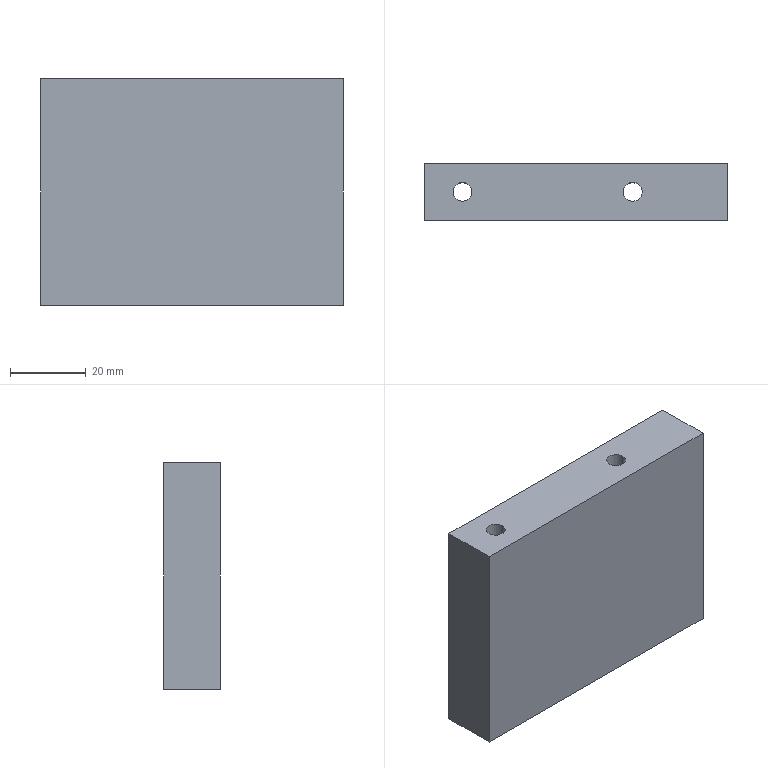Part | STEP file | PN_0025 | 1 solid | 10 faces | box 80 x 15 x 60 mm | volume 69644 mm3 | plane 6 | cylinder 4 | commonest cylinder face diameters 5 x4
STEP:
#1=CARTESIAN_POINT('',(0.,0.,0.));
#2=DIRECTION('',(0.,0.,1.));
#3=DIRECTION('',(1.,0.,0.));
#4=AXIS2_PLACEMENT_3D('',#1,#2,#3);
#5=CARTESIAN_POINT('',(-27.5,0.,-30.));
#6=VERTEX_POINT('',#5);
#7=CARTESIAN_POINT('',(-27.5,0.,30.));
#8=VERTEX_POINT('',#7);
#9=CARTESIAN_POINT('',(-27.5,0.,30.));
#10=DIRECTION('',(0.,0.,1.));
#11=VECTOR('',#10,1.);
#12=LINE('',#9,#11);
#13=CARTESIAN_POINT('',(-30.,0.,30.));
#14=DIRECTION('',(0.,0.,1.));
#15=DIRECTION('',(1.,0.,0.));
#16=AXIS2_PLACEMENT_3D('',#13,#14,#15);
#17=CYLINDRICAL_SURFACE('',#16,2.5);
#18=CARTESIAN_POINT('',(6.283,0.));
#19=DIRECTION('',(0.,1.));
#20=VECTOR('',#19,1.);
#21=LINE('',#18,#20);
#22=(GEOMETRIC_REPRESENTATION_CONTEXT(2)PARAMETRIC_REPRESENTATION_CONTEXT()REPRESENTATION_CONTEXT('',''));
#23=DEFINITIONAL_REPRESENTATION('',(#21),#22);
#24=PCURVE('',#17,#23);
#25=CARTESIAN_POINT('',(-30.,0.,30.));
#26=DIRECTION('',(0.,0.,1.));
#27=DIRECTION('',(1.,0.,0.));
#28=AXIS2_PLACEMENT_3D('',#25,#26,#27);
#29=CYLINDRICAL_SURFACE('',#28,2.5);
#30=CARTESIAN_POINT('',(0.,0.));
#31=DIRECTION('',(0.,1.));
#32=VECTOR('',#31,1.);
#33=LINE('',#30,#32);
#34=(GEOMETRIC_REPRESENTATION_CONTEXT(2)PARAMETRIC_REPRESENTATION_CONTEXT()REPRESENTATION_CONTEXT('',''));
#35=DEFINITIONAL_REPRESENTATION('',(#33),#34);
#36=PCURVE('',#29,#35);
#37=SURFACE_CURVE('',#12,(#24,#36),.PCURVE_S1.);
#38=EDGE_CURVE('',#6,#8,#37,.T.);
#39=ORIENTED_EDGE('',*,*,#38,.T.);
#40=CARTESIAN_POINT('',(-32.5,0.,30.));
#41=VERTEX_POINT('',#40);
#42=CARTESIAN_POINT('',(-30.,0.,30.));
#43=DIRECTION('',(0.,0.,1.));
#44=DIRECTION('',(1.,0.,0.));
#45=AXIS2_PLACEMENT_3D('',#42,#43,#44);
#46=CIRCLE('',#45,2.5);
#47=CARTESIAN_POINT('',(0.,0.));
#48=DIRECTION('',(1.,0.));
#49=VECTOR('',#48,1.);
#50=LINE('',#47,#49);
#51=(GEOMETRIC_REPRESENTATION_CONTEXT(2)PARAMETRIC_REPRESENTATION_CONTEXT()REPRESENTATION_CONTEXT('',''));
#52=DEFINITIONAL_REPRESENTATION('',(#50),#51);
#53=PCURVE('',#17,#52);
#54=CARTESIAN_POINT('',(-40.,7.5,30.));
#55=DIRECTION('',(0.,0.,-1.));
#56=DIRECTION('',(-1.,0.,0.));
#57=AXIS2_PLACEMENT_3D('',#54,#55,#56);
#58=PLANE('',#57);
#59=CARTESIAN_POINT('',(-12.5,-7.5));
#60=CARTESIAN_POINT('',(-12.5,-3.17));
#61=CARTESIAN_POINT('',(-8.75,-5.335));
#62=CARTESIAN_POINT('',(-5.,-7.5));
#63=CARTESIAN_POINT('',(-8.75,-9.665));
#64=CARTESIAN_POINT('',(-12.5,-11.83));
#65=CARTESIAN_POINT('',(-12.5,-7.5));
#66=(BOUNDED_CURVE()B_SPLINE_CURVE(2,(#59,#60,#61,#62,#63,#64,#65),.UNSPECIFIED.,.T.,.F.)B_SPLINE_CURVE_WITH_KNOTS((1,2,2,2,2,1),(-2.094,0.,2.094,4.189,6.283,8.378),.UNSPECIFIED.)CURVE()GEOMETRIC_REPRESENTATION_ITEM()RATIONAL_B_SPLINE_CURVE((1.,0.5,1.,0.5,1.,0.5,1.))REPRESENTATION_ITEM(''));
#67=(GEOMETRIC_REPRESENTATION_CONTEXT(2)PARAMETRIC_REPRESENTATION_CONTEXT()REPRESENTATION_CONTEXT('',''));
#68=DEFINITIONAL_REPRESENTATION('',(#66),#67);
#69=PCURVE('',#58,#68);
#70=SURFACE_CURVE('',#46,(#53,#69),.PCURVE_S1.);
#71=EDGE_CURVE('',#41,#8,#70,.T.);
#72=ORIENTED_EDGE('',*,*,#71,.F.);
#73=CARTESIAN_POINT('',(-32.5,0.,-30.));
#74=VERTEX_POINT('',#73);
#75=CARTESIAN_POINT('',(-32.5,0.,30.));
#76=DIRECTION('',(0.,0.,1.));
#77=VECTOR('',#76,1.);
#78=LINE('',#75,#77);
#79=CARTESIAN_POINT('',(3.142,0.));
#80=DIRECTION('',(0.,1.));
#81=VECTOR('',#80,1.);
#82=LINE('',#79,#81);
#83=(GEOMETRIC_REPRESENTATION_CONTEXT(2)PARAMETRIC_REPRESENTATION_CONTEXT()REPRESENTATION_CONTEXT('',''));
#84=DEFINITIONAL_REPRESENTATION('',(#82),#83);
#85=PCURVE('',#17,#84);
#86=CARTESIAN_POINT('',(3.142,0.));
#87=DIRECTION('',(0.,1.));
#88=VECTOR('',#87,1.);
#89=LINE('',#86,#88);
#90=(GEOMETRIC_REPRESENTATION_CONTEXT(2)PARAMETRIC_REPRESENTATION_CONTEXT()REPRESENTATION_CONTEXT('',''));
#91=DEFINITIONAL_REPRESENTATION('',(#89),#90);
#92=PCURVE('',#29,#91);
#93=SURFACE_CURVE('',#78,(#85,#92),.PCURVE_S1.);
#94=EDGE_CURVE('',#74,#41,#93,.T.);
#95=ORIENTED_EDGE('',*,*,#94,.F.);
#96=CARTESIAN_POINT('',(-30.,0.,-30.));
#97=DIRECTION('',(0.,0.,1.));
#98=DIRECTION('',(1.,0.,0.));
#99=AXIS2_PLACEMENT_3D('',#96,#97,#98);
#100=CIRCLE('',#99,2.5);
#101=CARTESIAN_POINT('',(0.,-60.));
#102=DIRECTION('',(1.,0.));
#103=VECTOR('',#102,1.);
#104=LINE('',#101,#103);
#105=(GEOMETRIC_REPRESENTATION_CONTEXT(2)PARAMETRIC_REPRESENTATION_CONTEXT()REPRESENTATION_CONTEXT('',''));
#106=DEFINITIONAL_REPRESENTATION('',(#104),#105);
#107=PCURVE('',#17,#106);
#108=CARTESIAN_POINT('',(-40.,7.5,-30.));
#109=DIRECTION('',(0.,0.,1.));
#110=DIRECTION('',(1.,0.,0.));
#111=AXIS2_PLACEMENT_3D('',#108,#109,#110);
#112=PLANE('',#111);
#113=CARTESIAN_POINT('',(10.,-7.5));
#114=DIRECTION('',(1.,0.));
#115=AXIS2_PLACEMENT_2D('',#113,#114);
#116=CIRCLE('',#115,2.5);
#117=(GEOMETRIC_REPRESENTATION_CONTEXT(2)PARAMETRIC_REPRESENTATION_CONTEXT()REPRESENTATION_CONTEXT('',''));
#118=DEFINITIONAL_REPRESENTATION('',(#116),#117);
#119=PCURVE('',#112,#118);
#120=SURFACE_CURVE('',#100,(#107,#119),.PCURVE_S1.);
#121=EDGE_CURVE('',#74,#6,#120,.T.);
#122=ORIENTED_EDGE('',*,*,#121,.T.);
#123=EDGE_LOOP('',(#39,#72,#95,#122));
#124=FACE_BOUND('',#123,.F.);
#125=ADVANCED_FACE('',(#124),#17,.F.);
#126=CARTESIAN_POINT('',(17.5,0.,-30.));
#127=VERTEX_POINT('',#126);
#128=CARTESIAN_POINT('',(17.5,0.,30.));
#129=VERTEX_POINT('',#128);
#130=CARTESIAN_POINT('',(17.5,0.,30.));
#131=DIRECTION('',(0.,0.,1.));
#132=VECTOR('',#131,1.);
#133=LINE('',#130,#132);
#134=CARTESIAN_POINT('',(15.,0.,30.));
#135=DIRECTION('',(0.,0.,1.));
#136=DIRECTION('',(1.,0.,0.));
#137=AXIS2_PLACEMENT_3D('',#134,#135,#136);
#138=CYLINDRICAL_SURFACE('',#137,2.5);
#139=CARTESIAN_POINT('',(6.283,0.));
#140=DIRECTION('',(0.,1.));
#141=VECTOR('',#140,1.);
#142=LINE('',#139,#141);
#143=(GEOMETRIC_REPRESENTATION_CONTEXT(2)PARAMETRIC_REPRESENTATION_CONTEXT()REPRESENTATION_CONTEXT('',''));
#144=DEFINITIONAL_REPRESENTATION('',(#142),#143);
#145=PCURVE('',#138,#144);
#146=CARTESIAN_POINT('',(15.,0.,30.));
#147=DIRECTION('',(0.,0.,1.));
#148=DIRECTION('',(1.,0.,0.));
#149=AXIS2_PLACEMENT_3D('',#146,#147,#148);
#150=CYLINDRICAL_SURFACE('',#149,2.5);
#151=CARTESIAN_POINT('',(0.,0.));
#152=DIRECTION('',(0.,1.));
#153=VECTOR('',#152,1.);
#154=LINE('',#151,#153);
#155=(GEOMETRIC_REPRESENTATION_CONTEXT(2)PARAMETRIC_REPRESENTATION_CONTEXT()REPRESENTATION_CONTEXT('',''));
#156=DEFINITIONAL_REPRESENTATION('',(#154),#155);
#157=PCURVE('',#150,#156);
#158=SURFACE_CURVE('',#133,(#145,#157),.PCURVE_S1.);
#159=EDGE_CURVE('',#127,#129,#158,.T.);
#160=ORIENTED_EDGE('',*,*,#159,.T.);
#161=CARTESIAN_POINT('',(12.5,0.,30.));
#162=VERTEX_POINT('',#161);
#163=CARTESIAN_POINT('',(15.,0.,30.));
#164=DIRECTION('',(0.,0.,1.));
#165=DIRECTION('',(1.,0.,0.));
#166=AXIS2_PLACEMENT_3D('',#163,#164,#165);
#167=CIRCLE('',#166,2.5);
#168=CARTESIAN_POINT('',(0.,0.));
#169=DIRECTION('',(1.,0.));
#170=VECTOR('',#169,1.);
#171=LINE('',#168,#170);
#172=(GEOMETRIC_REPRESENTATION_CONTEXT(2)PARAMETRIC_REPRESENTATION_CONTEXT()REPRESENTATION_CONTEXT('',''));
#173=DEFINITIONAL_REPRESENTATION('',(#171),#172);
#174=PCURVE('',#138,#173);
#175=CARTESIAN_POINT('',(-57.5,-7.5));
#176=CARTESIAN_POINT('',(-57.5,-3.17));
#177=CARTESIAN_POINT('',(-53.75,-5.335));
#178=CARTESIAN_POINT('',(-50.,-7.5));
#179=CARTESIAN_POINT('',(-53.75,-9.665));
#180=CARTESIAN_POINT('',(-57.5,-11.83));
#181=CARTESIAN_POINT('',(-57.5,-7.5));
#182=(BOUNDED_CURVE()B_SPLINE_CURVE(2,(#175,#176,#177,#178,#179,#180,#181),.UNSPECIFIED.,.T.,.F.)B_SPLINE_CURVE_WITH_KNOTS((1,2,2,2,2,1),(-2.094,0.,2.094,4.189,6.283,8.378),.UNSPECIFIED.)CURVE()GEOMETRIC_REPRESENTATION_ITEM()RATIONAL_B_SPLINE_CURVE((1.,0.5,1.,0.5,1.,0.5,1.))REPRESENTATION_ITEM(''));
#183=(GEOMETRIC_REPRESENTATION_CONTEXT(2)PARAMETRIC_REPRESENTATION_CONTEXT()REPRESENTATION_CONTEXT('',''));
#184=DEFINITIONAL_REPRESENTATION('',(#182),#183);
#185=PCURVE('',#58,#184);
#186=SURFACE_CURVE('',#167,(#174,#185),.PCURVE_S1.);
#187=EDGE_CURVE('',#162,#129,#186,.T.);
#188=ORIENTED_EDGE('',*,*,#187,.F.);
#189=CARTESIAN_POINT('',(12.5,0.,-30.));
#190=VERTEX_POINT('',#189);
#191=CARTESIAN_POINT('',(12.5,0.,30.));
#192=DIRECTION('',(0.,0.,1.));
#193=VECTOR('',#192,1.);
#194=LINE('',#191,#193);
#195=CARTESIAN_POINT('',(3.142,0.));
#196=DIRECTION('',(0.,1.));
#197=VECTOR('',#196,1.);
#198=LINE('',#195,#197);
#199=(GEOMETRIC_REPRESENTATION_CONTEXT(2)PARAMETRIC_REPRESENTATION_CONTEXT()REPRESENTATION_CONTEXT('',''));
#200=DEFINITIONAL_REPRESENTATION('',(#198),#199);
#201=PCURVE('',#138,#200);
#202=CARTESIAN_POINT('',(3.142,0.));
#203=DIRECTION('',(0.,1.));
#204=VECTOR('',#203,1.);
#205=LINE('',#202,#204);
#206=(GEOMETRIC_REPRESENTATION_CONTEXT(2)PARAMETRIC_REPRESENTATION_CONTEXT()REPRESENTATION_CONTEXT('',''));
#207=DEFINITIONAL_REPRESENTATION('',(#205),#206);
#208=PCURVE('',#150,#207);
#209=SURFACE_CURVE('',#194,(#201,#208),.PCURVE_S1.);
#210=EDGE_CURVE('',#190,#162,#209,.T.);
#211=ORIENTED_EDGE('',*,*,#210,.F.);
#212=CARTESIAN_POINT('',(15.,0.,-30.));
#213=DIRECTION('',(0.,0.,1.));
#214=DIRECTION('',(1.,0.,0.));
#215=AXIS2_PLACEMENT_3D('',#212,#213,#214);
#216=CIRCLE('',#215,2.5);
#217=CARTESIAN_POINT('',(0.,-60.));
#218=DIRECTION('',(1.,0.));
#219=VECTOR('',#218,1.);
#220=LINE('',#217,#219);
#221=(GEOMETRIC_REPRESENTATION_CONTEXT(2)PARAMETRIC_REPRESENTATION_CONTEXT()REPRESENTATION_CONTEXT('',''));
#222=DEFINITIONAL_REPRESENTATION('',(#220),#221);
#223=PCURVE('',#138,#222);
#224=CARTESIAN_POINT('',(55.,-7.5));
#225=DIRECTION('',(1.,0.));
#226=AXIS2_PLACEMENT_2D('',#224,#225);
#227=CIRCLE('',#226,2.5);
#228=(GEOMETRIC_REPRESENTATION_CONTEXT(2)PARAMETRIC_REPRESENTATION_CONTEXT()REPRESENTATION_CONTEXT('',''));
#229=DEFINITIONAL_REPRESENTATION('',(#227),#228);
#230=PCURVE('',#112,#229);
#231=SURFACE_CURVE('',#216,(#223,#230),.PCURVE_S1.);
#232=EDGE_CURVE('',#190,#127,#231,.T.);
#233=ORIENTED_EDGE('',*,*,#232,.T.);
#234=EDGE_LOOP('',(#160,#188,#211,#233));
#235=FACE_BOUND('',#234,.F.);
#236=ADVANCED_FACE('',(#235),#138,.F.);
#237=CARTESIAN_POINT('',(40.,-7.5,30.));
#238=VERTEX_POINT('',#237);
#239=CARTESIAN_POINT('',(40.,-7.5,-30.));
#240=VERTEX_POINT('',#239);
#241=CARTESIAN_POINT('',(40.,-7.5,-30.));
#242=DIRECTION('',(0.,0.,-1.));
#243=VECTOR('',#242,1.);
#244=LINE('',#241,#243);
#245=CARTESIAN_POINT('',(40.,7.5,-30.));
#246=DIRECTION('',(-1.,0.,0.));
#247=DIRECTION('',(0.,0.,1.));
#248=AXIS2_PLACEMENT_3D('',#245,#246,#247);
#249=PLANE('',#248);
#250=CARTESIAN_POINT('',(0.,-15.));
#251=DIRECTION('',(-1.,0.));
#252=VECTOR('',#251,1.);
#253=LINE('',#250,#252);
#254=(GEOMETRIC_REPRESENTATION_CONTEXT(2)PARAMETRIC_REPRESENTATION_CONTEXT()REPRESENTATION_CONTEXT('',''));
#255=DEFINITIONAL_REPRESENTATION('',(#253),#254);
#256=PCURVE('',#249,#255);
#257=CARTESIAN_POINT('',(0.,-7.5,0.));
#258=DIRECTION('',(0.,1.,0.));
#259=DIRECTION('',(0.,0.,1.));
#260=AXIS2_PLACEMENT_3D('',#257,#258,#259);
#261=PLANE('',#260);
#262=CARTESIAN_POINT('',(-30.,40.));
#263=DIRECTION('',(-1.,0.));
#264=VECTOR('',#263,1.);
#265=LINE('',#262,#264);
#266=(GEOMETRIC_REPRESENTATION_CONTEXT(2)PARAMETRIC_REPRESENTATION_CONTEXT()REPRESENTATION_CONTEXT('',''));
#267=DEFINITIONAL_REPRESENTATION('',(#265),#266);
#268=PCURVE('',#261,#267);
#269=SURFACE_CURVE('',#244,(#256,#268),.PCURVE_S1.);
#270=EDGE_CURVE('',#238,#240,#269,.T.);
#271=ORIENTED_EDGE('',*,*,#270,.T.);
#272=CARTESIAN_POINT('',(40.,7.5,-30.));
#273=VERTEX_POINT('',#272);
#274=CARTESIAN_POINT('',(40.,7.5,-30.));
#275=DIRECTION('',(0.,-1.,0.));
#276=VECTOR('',#275,1.);
#277=LINE('',#274,#276);
#278=CARTESIAN_POINT('',(0.,0.));
#279=DIRECTION('',(0.,-1.));
#280=VECTOR('',#279,1.);
#281=LINE('',#278,#280);
#282=(GEOMETRIC_REPRESENTATION_CONTEXT(2)PARAMETRIC_REPRESENTATION_CONTEXT()REPRESENTATION_CONTEXT('',''));
#283=DEFINITIONAL_REPRESENTATION('',(#281),#282);
#284=PCURVE('',#249,#283);
#285=CARTESIAN_POINT('',(80.,0.));
#286=DIRECTION('',(0.,-1.));
#287=VECTOR('',#286,1.);
#288=LINE('',#285,#287);
#289=(GEOMETRIC_REPRESENTATION_CONTEXT(2)PARAMETRIC_REPRESENTATION_CONTEXT()REPRESENTATION_CONTEXT('',''));
#290=DEFINITIONAL_REPRESENTATION('',(#288),#289);
#291=PCURVE('',#112,#290);
#292=SURFACE_CURVE('',#277,(#284,#291),.PCURVE_S1.);
#293=EDGE_CURVE('',#273,#240,#292,.T.);
#294=ORIENTED_EDGE('',*,*,#293,.F.);
#295=CARTESIAN_POINT('',(40.,7.5,30.));
#296=VERTEX_POINT('',#295);
#297=CARTESIAN_POINT('',(40.,7.5,-30.));
#298=DIRECTION('',(0.,0.,-1.));
#299=VECTOR('',#298,1.);
#300=LINE('',#297,#299);
#301=CARTESIAN_POINT('',(0.,0.));
#302=DIRECTION('',(-1.,0.));
#303=VECTOR('',#302,1.);
#304=LINE('',#301,#303);
#305=(GEOMETRIC_REPRESENTATION_CONTEXT(2)PARAMETRIC_REPRESENTATION_CONTEXT()REPRESENTATION_CONTEXT('',''));
#306=DEFINITIONAL_REPRESENTATION('',(#304),#305);
#307=PCURVE('',#249,#306);
#308=CARTESIAN_POINT('',(0.,7.5,0.));
#309=DIRECTION('',(0.,1.,0.));
#310=DIRECTION('',(0.,0.,1.));
#311=AXIS2_PLACEMENT_3D('',#308,#309,#310);
#312=PLANE('',#311);
#313=CARTESIAN_POINT('',(-30.,40.));
#314=DIRECTION('',(-1.,0.));
#315=VECTOR('',#314,1.);
#316=LINE('',#313,#315);
#317=(GEOMETRIC_REPRESENTATION_CONTEXT(2)PARAMETRIC_REPRESENTATION_CONTEXT()REPRESENTATION_CONTEXT('',''));
#318=DEFINITIONAL_REPRESENTATION('',(#316),#317);
#319=PCURVE('',#312,#318);
#320=SURFACE_CURVE('',#300,(#307,#319),.PCURVE_S1.);
#321=EDGE_CURVE('',#296,#273,#320,.T.);
#322=ORIENTED_EDGE('',*,*,#321,.F.);
#323=CARTESIAN_POINT('',(40.,7.5,30.));
#324=DIRECTION('',(0.,-1.,0.));
#325=VECTOR('',#324,1.);
#326=LINE('',#323,#325);
#327=CARTESIAN_POINT('',(60.,0.));
#328=DIRECTION('',(0.,-1.));
#329=VECTOR('',#328,1.);
#330=LINE('',#327,#329);
#331=(GEOMETRIC_REPRESENTATION_CONTEXT(2)PARAMETRIC_REPRESENTATION_CONTEXT()REPRESENTATION_CONTEXT('',''));
#332=DEFINITIONAL_REPRESENTATION('',(#330),#331);
#333=PCURVE('',#249,#332);
#334=CARTESIAN_POINT('',(-80.,0.));
#335=DIRECTION('',(0.,-1.));
#336=VECTOR('',#335,1.);
#337=LINE('',#334,#336);
#338=(GEOMETRIC_REPRESENTATION_CONTEXT(2)PARAMETRIC_REPRESENTATION_CONTEXT()REPRESENTATION_CONTEXT('',''));
#339=DEFINITIONAL_REPRESENTATION('',(#337),#338);
#340=PCURVE('',#58,#339);
#341=SURFACE_CURVE('',#326,(#333,#340),.PCURVE_S1.);
#342=EDGE_CURVE('',#296,#238,#341,.T.);
#343=ORIENTED_EDGE('',*,*,#342,.T.);
#344=EDGE_LOOP('',(#271,#294,#322,#343));
#345=FACE_BOUND('',#344,.T.);
#346=ADVANCED_FACE('',(#345),#249,.F.);
#347=CARTESIAN_POINT('',(-30.,0.,-30.));
#348=DIRECTION('',(0.,0.,1.));
#349=DIRECTION('',(1.,0.,0.));
#350=AXIS2_PLACEMENT_3D('',#347,#348,#349);
#351=CIRCLE('',#350,2.5);
#352=CARTESIAN_POINT('',(10.,-7.5));
#353=DIRECTION('',(1.,0.));
#354=AXIS2_PLACEMENT_2D('',#352,#353);
#355=CIRCLE('',#354,2.5);
#356=(GEOMETRIC_REPRESENTATION_CONTEXT(2)PARAMETRIC_REPRESENTATION_CONTEXT()REPRESENTATION_CONTEXT('',''));
#357=DEFINITIONAL_REPRESENTATION('',(#355),#356);
#358=PCURVE('',#112,#357);
#359=CARTESIAN_POINT('',(0.,-60.));
#360=DIRECTION('',(1.,0.));
#361=VECTOR('',#360,1.);
#362=LINE('',#359,#361);
#363=(GEOMETRIC_REPRESENTATION_CONTEXT(2)PARAMETRIC_REPRESENTATION_CONTEXT()REPRESENTATION_CONTEXT('',''));
#364=DEFINITIONAL_REPRESENTATION('',(#362),#363);
#365=PCURVE('',#29,#364);
#366=SURFACE_CURVE('',#351,(#358,#365),.PCURVE_S1.);
#367=EDGE_CURVE('',#6,#74,#366,.T.);
#368=ORIENTED_EDGE('',*,*,#367,.T.);
#369=ORIENTED_EDGE('',*,*,#121,.T.);
#370=EDGE_LOOP('',(#368,#369));
#371=FACE_BOUND('',#370,.T.);
#372=CARTESIAN_POINT('',(15.,0.,-30.));
#373=DIRECTION('',(0.,0.,1.));
#374=DIRECTION('',(1.,0.,0.));
#375=AXIS2_PLACEMENT_3D('',#372,#373,#374);
#376=CIRCLE('',#375,2.5);
#377=CARTESIAN_POINT('',(55.,-7.5));
#378=DIRECTION('',(1.,0.));
#379=AXIS2_PLACEMENT_2D('',#377,#378);
#380=CIRCLE('',#379,2.5);
#381=(GEOMETRIC_REPRESENTATION_CONTEXT(2)PARAMETRIC_REPRESENTATION_CONTEXT()REPRESENTATION_CONTEXT('',''));
#382=DEFINITIONAL_REPRESENTATION('',(#380),#381);
#383=PCURVE('',#112,#382);
#384=CARTESIAN_POINT('',(0.,-60.));
#385=DIRECTION('',(1.,0.));
#386=VECTOR('',#385,1.);
#387=LINE('',#384,#386);
#388=(GEOMETRIC_REPRESENTATION_CONTEXT(2)PARAMETRIC_REPRESENTATION_CONTEXT()REPRESENTATION_CONTEXT('',''));
#389=DEFINITIONAL_REPRESENTATION('',(#387),#388);
#390=PCURVE('',#150,#389);
#391=SURFACE_CURVE('',#376,(#383,#390),.PCURVE_S1.);
#392=EDGE_CURVE('',#127,#190,#391,.T.);
#393=ORIENTED_EDGE('',*,*,#392,.T.);
#394=ORIENTED_EDGE('',*,*,#232,.T.);
#395=EDGE_LOOP('',(#393,#394));
#396=FACE_BOUND('',#395,.T.);
#397=CARTESIAN_POINT('',(-40.,-7.5,-30.));
#398=VERTEX_POINT('',#397);
#399=CARTESIAN_POINT('',(-40.,-7.5,-30.));
#400=DIRECTION('',(-1.,0.,0.));
#401=VECTOR('',#400,1.);
#402=LINE('',#399,#401);
#403=CARTESIAN_POINT('',(0.,-15.));
#404=DIRECTION('',(-1.,0.));
#405=VECTOR('',#404,1.);
#406=LINE('',#403,#405);
#407=(GEOMETRIC_REPRESENTATION_CONTEXT(2)PARAMETRIC_REPRESENTATION_CONTEXT()REPRESENTATION_CONTEXT('',''));
#408=DEFINITIONAL_REPRESENTATION('',(#406),#407);
#409=PCURVE('',#112,#408);
#410=CARTESIAN_POINT('',(-30.,-40.));
#411=DIRECTION('',(0.,-1.));
#412=VECTOR('',#411,1.);
#413=LINE('',#410,#412);
#414=(GEOMETRIC_REPRESENTATION_CONTEXT(2)PARAMETRIC_REPRESENTATION_CONTEXT()REPRESENTATION_CONTEXT('',''));
#415=DEFINITIONAL_REPRESENTATION('',(#413),#414);
#416=PCURVE('',#261,#415);
#417=SURFACE_CURVE('',#402,(#409,#416),.PCURVE_S1.);
#418=EDGE_CURVE('',#240,#398,#417,.T.);
#419=ORIENTED_EDGE('',*,*,#418,.T.);
#420=CARTESIAN_POINT('',(-40.,7.5,-30.));
#421=VERTEX_POINT('',#420);
#422=CARTESIAN_POINT('',(-40.,7.5,-30.));
#423=DIRECTION('',(0.,-1.,0.));
#424=VECTOR('',#423,1.);
#425=LINE('',#422,#424);
#426=CARTESIAN_POINT('',(0.,0.));
#427=DIRECTION('',(0.,-1.));
#428=VECTOR('',#427,1.);
#429=LINE('',#426,#428);
#430=(GEOMETRIC_REPRESENTATION_CONTEXT(2)PARAMETRIC_REPRESENTATION_CONTEXT()REPRESENTATION_CONTEXT('',''));
#431=DEFINITIONAL_REPRESENTATION('',(#429),#430);
#432=PCURVE('',#112,#431);
#433=CARTESIAN_POINT('',(-40.,7.5,-30.));
#434=DIRECTION('',(1.,0.,0.));
#435=DIRECTION('',(0.,0.,-1.));
#436=AXIS2_PLACEMENT_3D('',#433,#434,#435);
#437=PLANE('',#436);
#438=CARTESIAN_POINT('',(0.,0.));
#439=DIRECTION('',(0.,-1.));
#440=VECTOR('',#439,1.);
#441=LINE('',#438,#440);
#442=(GEOMETRIC_REPRESENTATION_CONTEXT(2)PARAMETRIC_REPRESENTATION_CONTEXT()REPRESENTATION_CONTEXT('',''));
#443=DEFINITIONAL_REPRESENTATION('',(#441),#442);
#444=PCURVE('',#437,#443);
#445=SURFACE_CURVE('',#425,(#432,#444),.PCURVE_S1.);
#446=EDGE_CURVE('',#421,#398,#445,.T.);
#447=ORIENTED_EDGE('',*,*,#446,.F.);
#448=CARTESIAN_POINT('',(-40.,7.5,-30.));
#449=DIRECTION('',(-1.,0.,0.));
#450=VECTOR('',#449,1.);
#451=LINE('',#448,#450);
#452=CARTESIAN_POINT('',(0.,0.));
#453=DIRECTION('',(-1.,0.));
#454=VECTOR('',#453,1.);
#455=LINE('',#452,#454);
#456=(GEOMETRIC_REPRESENTATION_CONTEXT(2)PARAMETRIC_REPRESENTATION_CONTEXT()REPRESENTATION_CONTEXT('',''));
#457=DEFINITIONAL_REPRESENTATION('',(#455),#456);
#458=PCURVE('',#112,#457);
#459=CARTESIAN_POINT('',(-30.,-40.));
#460=DIRECTION('',(0.,-1.));
#461=VECTOR('',#460,1.);
#462=LINE('',#459,#461);
#463=(GEOMETRIC_REPRESENTATION_CONTEXT(2)PARAMETRIC_REPRESENTATION_CONTEXT()REPRESENTATION_CONTEXT('',''));
#464=DEFINITIONAL_REPRESENTATION('',(#462),#463);
#465=PCURVE('',#312,#464);
#466=SURFACE_CURVE('',#451,(#458,#465),.PCURVE_S1.);
#467=EDGE_CURVE('',#273,#421,#466,.T.);
#468=ORIENTED_EDGE('',*,*,#467,.F.);
#469=ORIENTED_EDGE('',*,*,#293,.T.);
#470=EDGE_LOOP('',(#419,#447,#468,#469));
#471=FACE_BOUND('',#470,.T.);
#472=ADVANCED_FACE('',(#371,#396,#471),#112,.F.);
#473=CARTESIAN_POINT('',(-40.,-7.5,30.));
#474=VERTEX_POINT('',#473);
#475=CARTESIAN_POINT('',(-40.,-7.5,-30.));
#476=DIRECTION('',(0.,0.,1.));
#477=VECTOR('',#476,1.);
#478=LINE('',#475,#477);
#479=CARTESIAN_POINT('',(0.,-15.));
#480=DIRECTION('',(-1.,0.));
#481=VECTOR('',#480,1.);
#482=LINE('',#479,#481);
#483=(GEOMETRIC_REPRESENTATION_CONTEXT(2)PARAMETRIC_REPRESENTATION_CONTEXT()REPRESENTATION_CONTEXT('',''));
#484=DEFINITIONAL_REPRESENTATION('',(#482),#483);
#485=PCURVE('',#437,#484);
#486=CARTESIAN_POINT('',(-30.,-40.));
#487=DIRECTION('',(1.,0.));
#488=VECTOR('',#487,1.);
#489=LINE('',#486,#488);
#490=(GEOMETRIC_REPRESENTATION_CONTEXT(2)PARAMETRIC_REPRESENTATION_CONTEXT()REPRESENTATION_CONTEXT('',''));
#491=DEFINITIONAL_REPRESENTATION('',(#489),#490);
#492=PCURVE('',#261,#491);
#493=SURFACE_CURVE('',#478,(#485,#492),.PCURVE_S1.);
#494=EDGE_CURVE('',#398,#474,#493,.T.);
#495=ORIENTED_EDGE('',*,*,#494,.T.);
#496=CARTESIAN_POINT('',(-40.,7.5,30.));
#497=VERTEX_POINT('',#496);
#498=CARTESIAN_POINT('',(-40.,7.5,30.));
#499=DIRECTION('',(0.,-1.,0.));
#500=VECTOR('',#499,1.);
#501=LINE('',#498,#500);
#502=CARTESIAN_POINT('',(-60.,0.));
#503=DIRECTION('',(0.,-1.));
#504=VECTOR('',#503,1.);
#505=LINE('',#502,#504);
#506=(GEOMETRIC_REPRESENTATION_CONTEXT(2)PARAMETRIC_REPRESENTATION_CONTEXT()REPRESENTATION_CONTEXT('',''));
#507=DEFINITIONAL_REPRESENTATION('',(#505),#506);
#508=PCURVE('',#437,#507);
#509=CARTESIAN_POINT('',(0.,0.));
#510=DIRECTION('',(0.,-1.));
#511=VECTOR('',#510,1.);
#512=LINE('',#509,#511);
#513=(GEOMETRIC_REPRESENTATION_CONTEXT(2)PARAMETRIC_REPRESENTATION_CONTEXT()REPRESENTATION_CONTEXT('',''));
#514=DEFINITIONAL_REPRESENTATION('',(#512),#513);
#515=PCURVE('',#58,#514);
#516=SURFACE_CURVE('',#501,(#508,#515),.PCURVE_S1.);
#517=EDGE_CURVE('',#497,#474,#516,.T.);
#518=ORIENTED_EDGE('',*,*,#517,.F.);
#519=CARTESIAN_POINT('',(-40.,7.5,-30.));
#520=DIRECTION('',(0.,0.,1.));
#521=VECTOR('',#520,1.);
#522=LINE('',#519,#521);
#523=CARTESIAN_POINT('',(0.,0.));
#524=DIRECTION('',(-1.,0.));
#525=VECTOR('',#524,1.);
#526=LINE('',#523,#525);
#527=(GEOMETRIC_REPRESENTATION_CONTEXT(2)PARAMETRIC_REPRESENTATION_CONTEXT()REPRESENTATION_CONTEXT('',''));
#528=DEFINITIONAL_REPRESENTATION('',(#526),#527);
#529=PCURVE('',#437,#528);
#530=CARTESIAN_POINT('',(-30.,-40.));
#531=DIRECTION('',(1.,0.));
#532=VECTOR('',#531,1.);
#533=LINE('',#530,#532);
#534=(GEOMETRIC_REPRESENTATION_CONTEXT(2)PARAMETRIC_REPRESENTATION_CONTEXT()REPRESENTATION_CONTEXT('',''));
#535=DEFINITIONAL_REPRESENTATION('',(#533),#534);
#536=PCURVE('',#312,#535);
#537=SURFACE_CURVE('',#522,(#529,#536),.PCURVE_S1.);
#538=EDGE_CURVE('',#421,#497,#537,.T.);
#539=ORIENTED_EDGE('',*,*,#538,.F.);
#540=ORIENTED_EDGE('',*,*,#446,.T.);
#541=EDGE_LOOP('',(#495,#518,#539,#540));
#542=FACE_BOUND('',#541,.T.);
#543=ADVANCED_FACE('',(#542),#437,.F.);
#544=CARTESIAN_POINT('',(-30.,0.,30.));
#545=DIRECTION('',(0.,0.,1.));
#546=DIRECTION('',(1.,0.,0.));
#547=AXIS2_PLACEMENT_3D('',#544,#545,#546);
#548=CIRCLE('',#547,2.5);
#549=CARTESIAN_POINT('',(-12.5,-7.5));
#550=CARTESIAN_POINT('',(-12.5,-3.17));
#551=CARTESIAN_POINT('',(-8.75,-5.335));
#552=CARTESIAN_POINT('',(-5.,-7.5));
#553=CARTESIAN_POINT('',(-8.75,-9.665));
#554=CARTESIAN_POINT('',(-12.5,-11.83));
#555=CARTESIAN_POINT('',(-12.5,-7.5));
#556=(BOUNDED_CURVE()B_SPLINE_CURVE(2,(#549,#550,#551,#552,#553,#554,#555),.UNSPECIFIED.,.T.,.F.)B_SPLINE_CURVE_WITH_KNOTS((1,2,2,2,2,1),(-2.094,0.,2.094,4.189,6.283,8.378),.UNSPECIFIED.)CURVE()GEOMETRIC_REPRESENTATION_ITEM()RATIONAL_B_SPLINE_CURVE((1.,0.5,1.,0.5,1.,0.5,1.))REPRESENTATION_ITEM(''));
#557=(GEOMETRIC_REPRESENTATION_CONTEXT(2)PARAMETRIC_REPRESENTATION_CONTEXT()REPRESENTATION_CONTEXT('',''));
#558=DEFINITIONAL_REPRESENTATION('',(#556),#557);
#559=PCURVE('',#58,#558);
#560=CARTESIAN_POINT('',(0.,0.));
#561=DIRECTION('',(1.,0.));
#562=VECTOR('',#561,1.);
#563=LINE('',#560,#562);
#564=(GEOMETRIC_REPRESENTATION_CONTEXT(2)PARAMETRIC_REPRESENTATION_CONTEXT()REPRESENTATION_CONTEXT('',''));
#565=DEFINITIONAL_REPRESENTATION('',(#563),#564);
#566=PCURVE('',#29,#565);
#567=SURFACE_CURVE('',#548,(#559,#566),.PCURVE_S1.);
#568=EDGE_CURVE('',#8,#41,#567,.T.);
#569=ORIENTED_EDGE('',*,*,#568,.F.);
#570=ORIENTED_EDGE('',*,*,#71,.F.);
#571=EDGE_LOOP('',(#569,#570));
#572=FACE_BOUND('',#571,.T.);
#573=CARTESIAN_POINT('',(15.,0.,30.));
#574=DIRECTION('',(0.,0.,1.));
#575=DIRECTION('',(1.,0.,0.));
#576=AXIS2_PLACEMENT_3D('',#573,#574,#575);
#577=CIRCLE('',#576,2.5);
#578=CARTESIAN_POINT('',(-57.5,-7.5));
#579=CARTESIAN_POINT('',(-57.5,-3.17));
#580=CARTESIAN_POINT('',(-53.75,-5.335));
#581=CARTESIAN_POINT('',(-50.,-7.5));
#582=CARTESIAN_POINT('',(-53.75,-9.665));
#583=CARTESIAN_POINT('',(-57.5,-11.83));
#584=CARTESIAN_POINT('',(-57.5,-7.5));
#585=(BOUNDED_CURVE()B_SPLINE_CURVE(2,(#578,#579,#580,#581,#582,#583,#584),.UNSPECIFIED.,.T.,.F.)B_SPLINE_CURVE_WITH_KNOTS((1,2,2,2,2,1),(-2.094,0.,2.094,4.189,6.283,8.378),.UNSPECIFIED.)CURVE()GEOMETRIC_REPRESENTATION_ITEM()RATIONAL_B_SPLINE_CURVE((1.,0.5,1.,0.5,1.,0.5,1.))REPRESENTATION_ITEM(''));
#586=(GEOMETRIC_REPRESENTATION_CONTEXT(2)PARAMETRIC_REPRESENTATION_CONTEXT()REPRESENTATION_CONTEXT('',''));
#587=DEFINITIONAL_REPRESENTATION('',(#585),#586);
#588=PCURVE('',#58,#587);
#589=CARTESIAN_POINT('',(0.,0.));
#590=DIRECTION('',(1.,0.));
#591=VECTOR('',#590,1.);
#592=LINE('',#589,#591);
#593=(GEOMETRIC_REPRESENTATION_CONTEXT(2)PARAMETRIC_REPRESENTATION_CONTEXT()REPRESENTATION_CONTEXT('',''));
#594=DEFINITIONAL_REPRESENTATION('',(#592),#593);
#595=PCURVE('',#150,#594);
#596=SURFACE_CURVE('',#577,(#588,#595),.PCURVE_S1.);
#597=EDGE_CURVE('',#129,#162,#596,.T.);
#598=ORIENTED_EDGE('',*,*,#597,.F.);
#599=ORIENTED_EDGE('',*,*,#187,.F.);
#600=EDGE_LOOP('',(#598,#599));
#601=FACE_BOUND('',#600,.T.);
#602=CARTESIAN_POINT('',(-40.,-7.5,30.));
#603=DIRECTION('',(1.,0.,0.));
#604=VECTOR('',#603,1.);
#605=LINE('',#602,#604);
#606=CARTESIAN_POINT('',(0.,-15.));
#607=DIRECTION('',(-1.,0.));
#608=VECTOR('',#607,1.);
#609=LINE('',#606,#608);
#610=(GEOMETRIC_REPRESENTATION_CONTEXT(2)PARAMETRIC_REPRESENTATION_CONTEXT()REPRESENTATION_CONTEXT('',''));
#611=DEFINITIONAL_REPRESENTATION('',(#609),#610);
#612=PCURVE('',#58,#611);
#613=CARTESIAN_POINT('',(30.,-40.));
#614=DIRECTION('',(0.,1.));
#615=VECTOR('',#614,1.);
#616=LINE('',#613,#615);
#617=(GEOMETRIC_REPRESENTATION_CONTEXT(2)PARAMETRIC_REPRESENTATION_CONTEXT()REPRESENTATION_CONTEXT('',''));
#618=DEFINITIONAL_REPRESENTATION('',(#616),#617);
#619=PCURVE('',#261,#618);
#620=SURFACE_CURVE('',#605,(#612,#619),.PCURVE_S1.);
#621=EDGE_CURVE('',#474,#238,#620,.T.);
#622=ORIENTED_EDGE('',*,*,#621,.T.);
#623=ORIENTED_EDGE('',*,*,#342,.F.);
#624=CARTESIAN_POINT('',(-40.,7.5,30.));
#625=DIRECTION('',(1.,0.,0.));
#626=VECTOR('',#625,1.);
#627=LINE('',#624,#626);
#628=CARTESIAN_POINT('',(0.,0.));
#629=DIRECTION('',(-1.,0.));
#630=VECTOR('',#629,1.);
#631=LINE('',#628,#630);
#632=(GEOMETRIC_REPRESENTATION_CONTEXT(2)PARAMETRIC_REPRESENTATION_CONTEXT()REPRESENTATION_CONTEXT('',''));
#633=DEFINITIONAL_REPRESENTATION('',(#631),#632);
#634=PCURVE('',#58,#633);
#635=CARTESIAN_POINT('',(30.,-40.));
#636=DIRECTION('',(0.,1.));
#637=VECTOR('',#636,1.);
#638=LINE('',#635,#637);
#639=(GEOMETRIC_REPRESENTATION_CONTEXT(2)PARAMETRIC_REPRESENTATION_CONTEXT()REPRESENTATION_CONTEXT('',''));
#640=DEFINITIONAL_REPRESENTATION('',(#638),#639);
#641=PCURVE('',#312,#640);
#642=SURFACE_CURVE('',#627,(#634,#641),.PCURVE_S1.);
#643=EDGE_CURVE('',#497,#296,#642,.T.);
#644=ORIENTED_EDGE('',*,*,#643,.F.);
#645=ORIENTED_EDGE('',*,*,#517,.T.);
#646=EDGE_LOOP('',(#622,#623,#644,#645));
#647=FACE_BOUND('',#646,.T.);
#648=ADVANCED_FACE('',(#572,#601,#647),#58,.F.);
#649=ORIENTED_EDGE('',*,*,#321,.T.);
#650=ORIENTED_EDGE('',*,*,#467,.T.);
#651=ORIENTED_EDGE('',*,*,#538,.T.);
#652=ORIENTED_EDGE('',*,*,#643,.T.);
#653=EDGE_LOOP('',(#649,#650,#651,#652));
#654=FACE_BOUND('',#653,.T.);
#655=ADVANCED_FACE('',(#654),#312,.T.);
#656=ORIENTED_EDGE('',*,*,#270,.F.);
#657=ORIENTED_EDGE('',*,*,#621,.F.);
#658=ORIENTED_EDGE('',*,*,#494,.F.);
#659=ORIENTED_EDGE('',*,*,#418,.F.);
#660=EDGE_LOOP('',(#656,#657,#658,#659));
#661=FACE_BOUND('',#660,.T.);
#662=ADVANCED_FACE('',(#661),#261,.F.);
#663=ORIENTED_EDGE('',*,*,#597,.F.);
#664=ORIENTED_EDGE('',*,*,#159,.F.);
#665=ORIENTED_EDGE('',*,*,#392,.T.);
#666=ORIENTED_EDGE('',*,*,#210,.T.);
#667=EDGE_LOOP('',(#663,#664,#665,#666));
#668=FACE_BOUND('',#667,.F.);
#669=ADVANCED_FACE('',(#668),#150,.F.);
#670=ORIENTED_EDGE('',*,*,#568,.F.);
#671=ORIENTED_EDGE('',*,*,#38,.F.);
#672=ORIENTED_EDGE('',*,*,#367,.T.);
#673=ORIENTED_EDGE('',*,*,#94,.T.);
#674=EDGE_LOOP('',(#670,#671,#672,#673));
#675=FACE_BOUND('',#674,.F.);
#676=ADVANCED_FACE('',(#675),#29,.F.);
#677=CLOSED_SHELL('',(#125,#236,#346,#472,#543,#648,#655,#662,#669,#676));
#678=MANIFOLD_SOLID_BREP('',#677);
#679=(LENGTH_UNIT()NAMED_UNIT(*)SI_UNIT(.MILLI.,.METRE.));
#680=UNCERTAINTY_MEASURE_WITH_UNIT(LENGTH_MEASURE(0.0000001),#679,'','');
#681=(NAMED_UNIT(*)PLANE_ANGLE_UNIT()SI_UNIT($,.RADIAN.));
#682=(NAMED_UNIT(*)SI_UNIT($,.STERADIAN.)SOLID_ANGLE_UNIT());
#683=(GEOMETRIC_REPRESENTATION_CONTEXT(3)GLOBAL_UNCERTAINTY_ASSIGNED_CONTEXT((#680))GLOBAL_UNIT_ASSIGNED_CONTEXT((#679,#681,#682))REPRESENTATION_CONTEXT('',''));
#684=ADVANCED_BREP_SHAPE_REPRESENTATION('',(#4,#678),#683);